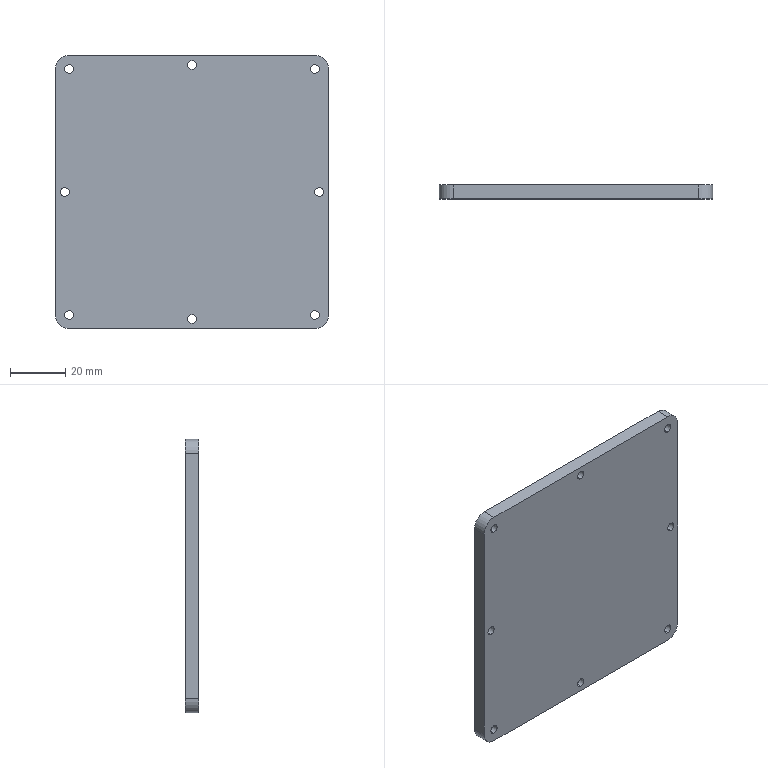Part | SolidWorks | features Extrusion 1, Fillet 1, HoleWzd 1 | 1 solid | 42 faces | box 99 x 5 x 99 mm | volume 48448 mm3 | cylinder 20 | cone 16 | plane 6 | commonest cylinder face diameters 3.2 x16 10 x4
STEP:
#1=CARTESIAN_POINT('',(-44.5,3.45,-46.1));
#2=VERTEX_POINT('',#1);
#3=CARTESIAN_POINT('',(-44.5,3.45,-42.9));
#4=VERTEX_POINT('',#3);
#5=CARTESIAN_POINT('',(-44.5,3.45,-44.5));
#6=DIRECTION('',(0.,1.,0.));
#7=DIRECTION('',(0.,0.,1.));
#8=AXIS2_PLACEMENT_3D('',#5,#6,#7);
#9=CIRCLE('',#8,1.6);
#10=EDGE_CURVE('',#2,#4,#9,.T.);
#11=ORIENTED_EDGE('',*,*,#10,.F.);
#12=CARTESIAN_POINT('',(-44.5,5.,-47.65));
#13=VERTEX_POINT('',#12);
#14=CARTESIAN_POINT('',(-44.5,5.,-47.65));
#15=DIRECTION('',(0.,0.7071,-0.7071));
#16=VECTOR('',#15,1000.);
#17=LINE('',#14,#16);
#18=EDGE_CURVE('',#2,#13,#17,.T.);
#19=ORIENTED_EDGE('',*,*,#18,.T.);
#20=CARTESIAN_POINT('',(-44.5,5.,-41.35));
#21=VERTEX_POINT('',#20);
#22=CARTESIAN_POINT('',(-44.5,5.,-44.5));
#23=DIRECTION('',(0.,1.,0.));
#24=DIRECTION('',(0.,0.,1.));
#25=AXIS2_PLACEMENT_3D('',#22,#23,#24);
#26=CIRCLE('',#25,3.15);
#27=EDGE_CURVE('',#13,#21,#26,.T.);
#28=ORIENTED_EDGE('',*,*,#27,.T.);
#29=CARTESIAN_POINT('',(-44.5,5.,-41.35));
#30=DIRECTION('',(0.,0.7071,0.7071));
#31=VECTOR('',#30,1000.);
#32=LINE('',#29,#31);
#33=EDGE_CURVE('',#4,#21,#32,.T.);
#34=ORIENTED_EDGE('',*,*,#33,.F.);
#35=EDGE_LOOP('',(#11,#19,#28,#34));
#36=FACE_OUTER_BOUND('',#35,.T.);
#37=CARTESIAN_POINT('',(-44.5,5.,-44.5));
#38=DIRECTION('',(0.,1.,0.));
#39=DIRECTION('',(0.,0.,1.));
#40=AXIS2_PLACEMENT_3D('',#37,#38,#39);
#41=CONICAL_SURFACE('',#40,3.15,0.7854);
#42=ADVANCED_FACE('',(#36),#41,.F.);
#43=CARTESIAN_POINT('',(-44.5,0.,-42.9));
#44=VERTEX_POINT('',#43);
#45=CARTESIAN_POINT('',(-44.5,0.,-46.1));
#46=VERTEX_POINT('',#45);
#47=CARTESIAN_POINT('',(-44.5,0.,-44.5));
#48=DIRECTION('',(0.,-1.,0.));
#49=DIRECTION('',(0.,0.,-1.));
#50=AXIS2_PLACEMENT_3D('',#47,#48,#49);
#51=CIRCLE('',#50,1.6);
#52=EDGE_CURVE('',#44,#46,#51,.T.);
#53=ORIENTED_EDGE('',*,*,#52,.T.);
#54=CARTESIAN_POINT('',(-44.5,5.,-46.1));
#55=DIRECTION('',(0.,1.,0.));
#56=VECTOR('',#55,1000.);
#57=LINE('',#54,#56);
#58=EDGE_CURVE('',#46,#2,#57,.T.);
#59=ORIENTED_EDGE('',*,*,#58,.T.);
#60=ORIENTED_EDGE('',*,*,#10,.T.);
#61=CARTESIAN_POINT('',(-44.5,5.,-42.9));
#62=DIRECTION('',(0.,1.,0.));
#63=VECTOR('',#62,1000.);
#64=LINE('',#61,#63);
#65=EDGE_CURVE('',#44,#4,#64,.T.);
#66=ORIENTED_EDGE('',*,*,#65,.F.);
#67=EDGE_LOOP('',(#53,#59,#60,#66));
#68=FACE_OUTER_BOUND('',#67,.T.);
#69=CARTESIAN_POINT('',(-44.5,5.,-44.5));
#70=DIRECTION('',(0.,1.,0.));
#71=DIRECTION('',(0.,0.,1.));
#72=AXIS2_PLACEMENT_3D('',#69,#70,#71);
#73=CYLINDRICAL_SURFACE('',#72,1.6);
#74=ADVANCED_FACE('',(#68),#73,.F.);
#75=CARTESIAN_POINT('',(44.5,3.45,-46.1));
#76=VERTEX_POINT('',#75);
#77=CARTESIAN_POINT('',(44.5,3.45,-42.9));
#78=VERTEX_POINT('',#77);
#79=CARTESIAN_POINT('',(44.5,3.45,-44.5));
#80=DIRECTION('',(0.,1.,0.));
#81=DIRECTION('',(0.,0.,1.));
#82=AXIS2_PLACEMENT_3D('',#79,#80,#81);
#83=CIRCLE('',#82,1.6);
#84=EDGE_CURVE('',#76,#78,#83,.T.);
#85=ORIENTED_EDGE('',*,*,#84,.F.);
#86=CARTESIAN_POINT('',(44.5,5.,-47.65));
#87=VERTEX_POINT('',#86);
#88=CARTESIAN_POINT('',(44.5,5.,-47.65));
#89=DIRECTION('',(0.,0.7071,-0.7071));
#90=VECTOR('',#89,1000.);
#91=LINE('',#88,#90);
#92=EDGE_CURVE('',#76,#87,#91,.T.);
#93=ORIENTED_EDGE('',*,*,#92,.T.);
#94=CARTESIAN_POINT('',(44.5,5.,-41.35));
#95=VERTEX_POINT('',#94);
#96=CARTESIAN_POINT('',(44.5,5.,-44.5));
#97=DIRECTION('',(0.,1.,0.));
#98=DIRECTION('',(0.,0.,1.));
#99=AXIS2_PLACEMENT_3D('',#96,#97,#98);
#100=CIRCLE('',#99,3.15);
#101=EDGE_CURVE('',#87,#95,#100,.T.);
#102=ORIENTED_EDGE('',*,*,#101,.T.);
#103=CARTESIAN_POINT('',(44.5,5.,-41.35));
#104=DIRECTION('',(0.,0.7071,0.7071));
#105=VECTOR('',#104,1000.);
#106=LINE('',#103,#105);
#107=EDGE_CURVE('',#78,#95,#106,.T.);
#108=ORIENTED_EDGE('',*,*,#107,.F.);
#109=EDGE_LOOP('',(#85,#93,#102,#108));
#110=FACE_OUTER_BOUND('',#109,.T.);
#111=CARTESIAN_POINT('',(44.5,5.,-44.5));
#112=DIRECTION('',(0.,1.,0.));
#113=DIRECTION('',(0.,0.,1.));
#114=AXIS2_PLACEMENT_3D('',#111,#112,#113);
#115=CONICAL_SURFACE('',#114,3.15,0.7854);
#116=ADVANCED_FACE('',(#110),#115,.F.);
#117=CARTESIAN_POINT('',(44.5,0.,-42.9));
#118=VERTEX_POINT('',#117);
#119=CARTESIAN_POINT('',(44.5,0.,-46.1));
#120=VERTEX_POINT('',#119);
#121=CARTESIAN_POINT('',(44.5,0.,-44.5));
#122=DIRECTION('',(0.,-1.,0.));
#123=DIRECTION('',(0.,0.,-1.));
#124=AXIS2_PLACEMENT_3D('',#121,#122,#123);
#125=CIRCLE('',#124,1.6);
#126=EDGE_CURVE('',#118,#120,#125,.T.);
#127=ORIENTED_EDGE('',*,*,#126,.T.);
#128=CARTESIAN_POINT('',(44.5,5.,-46.1));
#129=DIRECTION('',(0.,1.,0.));
#130=VECTOR('',#129,1000.);
#131=LINE('',#128,#130);
#132=EDGE_CURVE('',#120,#76,#131,.T.);
#133=ORIENTED_EDGE('',*,*,#132,.T.);
#134=ORIENTED_EDGE('',*,*,#84,.T.);
#135=CARTESIAN_POINT('',(44.5,5.,-42.9));
#136=DIRECTION('',(0.,1.,0.));
#137=VECTOR('',#136,1000.);
#138=LINE('',#135,#137);
#139=EDGE_CURVE('',#118,#78,#138,.T.);
#140=ORIENTED_EDGE('',*,*,#139,.F.);
#141=EDGE_LOOP('',(#127,#133,#134,#140));
#142=FACE_OUTER_BOUND('',#141,.T.);
#143=CARTESIAN_POINT('',(44.5,5.,-44.5));
#144=DIRECTION('',(0.,1.,0.));
#145=DIRECTION('',(0.,0.,1.));
#146=AXIS2_PLACEMENT_3D('',#143,#144,#145);
#147=CYLINDRICAL_SURFACE('',#146,1.6);
#148=ADVANCED_FACE('',(#142),#147,.F.);
#149=CARTESIAN_POINT('',(0.,3.45,-47.6));
#150=VERTEX_POINT('',#149);
#151=CARTESIAN_POINT('',(0.,3.45,-44.4));
#152=VERTEX_POINT('',#151);
#153=CARTESIAN_POINT('',(0.,3.45,-46.));
#154=DIRECTION('',(0.,1.,0.));
#155=DIRECTION('',(0.,0.,1.));
#156=AXIS2_PLACEMENT_3D('',#153,#154,#155);
#157=CIRCLE('',#156,1.6);
#158=EDGE_CURVE('',#150,#152,#157,.T.);
#159=ORIENTED_EDGE('',*,*,#158,.F.);
#160=CARTESIAN_POINT('',(0.,5.,-49.15));
#161=VERTEX_POINT('',#160);
#162=CARTESIAN_POINT('',(0.,5.,-49.15));
#163=DIRECTION('',(0.,0.7071,-0.7071));
#164=VECTOR('',#163,1000.);
#165=LINE('',#162,#164);
#166=EDGE_CURVE('',#150,#161,#165,.T.);
#167=ORIENTED_EDGE('',*,*,#166,.T.);
#168=CARTESIAN_POINT('',(0.,5.,-42.85));
#169=VERTEX_POINT('',#168);
#170=CARTESIAN_POINT('',(0.,5.,-46.));
#171=DIRECTION('',(0.,1.,0.));
#172=DIRECTION('',(0.,0.,1.));
#173=AXIS2_PLACEMENT_3D('',#170,#171,#172);
#174=CIRCLE('',#173,3.15);
#175=EDGE_CURVE('',#161,#169,#174,.T.);
#176=ORIENTED_EDGE('',*,*,#175,.T.);
#177=CARTESIAN_POINT('',(0.,5.,-42.85));
#178=DIRECTION('',(0.,0.7071,0.7071));
#179=VECTOR('',#178,1000.);
#180=LINE('',#177,#179);
#181=EDGE_CURVE('',#152,#169,#180,.T.);
#182=ORIENTED_EDGE('',*,*,#181,.F.);
#183=EDGE_LOOP('',(#159,#167,#176,#182));
#184=FACE_OUTER_BOUND('',#183,.T.);
#185=CARTESIAN_POINT('',(0.,5.,-46.));
#186=DIRECTION('',(0.,1.,0.));
#187=DIRECTION('',(0.,0.,1.));
#188=AXIS2_PLACEMENT_3D('',#185,#186,#187);
#189=CONICAL_SURFACE('',#188,3.15,0.7854);
#190=ADVANCED_FACE('',(#184),#189,.F.);
#191=CARTESIAN_POINT('',(0.,0.,-44.4));
#192=VERTEX_POINT('',#191);
#193=CARTESIAN_POINT('',(0.,0.,-47.6));
#194=VERTEX_POINT('',#193);
#195=CARTESIAN_POINT('',(0.,0.,-46.));
#196=DIRECTION('',(0.,-1.,0.));
#197=DIRECTION('',(0.,0.,-1.));
#198=AXIS2_PLACEMENT_3D('',#195,#196,#197);
#199=CIRCLE('',#198,1.6);
#200=EDGE_CURVE('',#192,#194,#199,.T.);
#201=ORIENTED_EDGE('',*,*,#200,.T.);
#202=CARTESIAN_POINT('',(0.,5.,-47.6));
#203=DIRECTION('',(0.,1.,0.));
#204=VECTOR('',#203,1000.);
#205=LINE('',#202,#204);
#206=EDGE_CURVE('',#194,#150,#205,.T.);
#207=ORIENTED_EDGE('',*,*,#206,.T.);
#208=ORIENTED_EDGE('',*,*,#158,.T.);
#209=CARTESIAN_POINT('',(0.,5.,-44.4));
#210=DIRECTION('',(0.,1.,0.));
#211=VECTOR('',#210,1000.);
#212=LINE('',#209,#211);
#213=EDGE_CURVE('',#192,#152,#212,.T.);
#214=ORIENTED_EDGE('',*,*,#213,.F.);
#215=EDGE_LOOP('',(#201,#207,#208,#214));
#216=FACE_OUTER_BOUND('',#215,.T.);
#217=CARTESIAN_POINT('',(0.,5.,-46.));
#218=DIRECTION('',(0.,1.,0.));
#219=DIRECTION('',(0.,0.,1.));
#220=AXIS2_PLACEMENT_3D('',#217,#218,#219);
#221=CYLINDRICAL_SURFACE('',#220,1.6);
#222=ADVANCED_FACE('',(#216),#221,.F.);
#223=CARTESIAN_POINT('',(-46.,3.45,-1.6));
#224=VERTEX_POINT('',#223);
#225=CARTESIAN_POINT('',(-46.,3.45,1.6));
#226=VERTEX_POINT('',#225);
#227=CARTESIAN_POINT('',(-46.,3.45,0.));
#228=DIRECTION('',(0.,1.,0.));
#229=DIRECTION('',(0.,0.,1.));
#230=AXIS2_PLACEMENT_3D('',#227,#228,#229);
#231=CIRCLE('',#230,1.6);
#232=EDGE_CURVE('',#224,#226,#231,.T.);
#233=ORIENTED_EDGE('',*,*,#232,.F.);
#234=CARTESIAN_POINT('',(-46.,5.,-3.15));
#235=VERTEX_POINT('',#234);
#236=CARTESIAN_POINT('',(-46.,5.,-3.15));
#237=DIRECTION('',(0.,0.7071,-0.7071));
#238=VECTOR('',#237,1000.);
#239=LINE('',#236,#238);
#240=EDGE_CURVE('',#224,#235,#239,.T.);
#241=ORIENTED_EDGE('',*,*,#240,.T.);
#242=CARTESIAN_POINT('',(-46.,5.,3.15));
#243=VERTEX_POINT('',#242);
#244=CARTESIAN_POINT('',(-46.,5.,0.));
#245=DIRECTION('',(0.,1.,0.));
#246=DIRECTION('',(0.,0.,1.));
#247=AXIS2_PLACEMENT_3D('',#244,#245,#246);
#248=CIRCLE('',#247,3.15);
#249=EDGE_CURVE('',#235,#243,#248,.T.);
#250=ORIENTED_EDGE('',*,*,#249,.T.);
#251=CARTESIAN_POINT('',(-46.,5.,3.15));
#252=DIRECTION('',(0.,0.7071,0.7071));
#253=VECTOR('',#252,1000.);
#254=LINE('',#251,#253);
#255=EDGE_CURVE('',#226,#243,#254,.T.);
#256=ORIENTED_EDGE('',*,*,#255,.F.);
#257=EDGE_LOOP('',(#233,#241,#250,#256));
#258=FACE_OUTER_BOUND('',#257,.T.);
#259=CARTESIAN_POINT('',(-46.,5.,0.));
#260=DIRECTION('',(0.,1.,0.));
#261=DIRECTION('',(0.,0.,1.));
#262=AXIS2_PLACEMENT_3D('',#259,#260,#261);
#263=CONICAL_SURFACE('',#262,3.15,0.7854);
#264=ADVANCED_FACE('',(#258),#263,.F.);
#265=CARTESIAN_POINT('',(-46.,0.,1.6));
#266=VERTEX_POINT('',#265);
#267=CARTESIAN_POINT('',(-46.,0.,-1.6));
#268=VERTEX_POINT('',#267);
#269=CARTESIAN_POINT('',(-46.,0.,0.));
#270=DIRECTION('',(0.,-1.,0.));
#271=DIRECTION('',(0.,0.,-1.));
#272=AXIS2_PLACEMENT_3D('',#269,#270,#271);
#273=CIRCLE('',#272,1.6);
#274=EDGE_CURVE('',#266,#268,#273,.T.);
#275=ORIENTED_EDGE('',*,*,#274,.T.);
#276=CARTESIAN_POINT('',(-46.,5.,-1.6));
#277=DIRECTION('',(0.,1.,0.));
#278=VECTOR('',#277,1000.);
#279=LINE('',#276,#278);
#280=EDGE_CURVE('',#268,#224,#279,.T.);
#281=ORIENTED_EDGE('',*,*,#280,.T.);
#282=ORIENTED_EDGE('',*,*,#232,.T.);
#283=CARTESIAN_POINT('',(-46.,5.,1.6));
#284=DIRECTION('',(0.,1.,0.));
#285=VECTOR('',#284,1000.);
#286=LINE('',#283,#285);
#287=EDGE_CURVE('',#266,#226,#286,.T.);
#288=ORIENTED_EDGE('',*,*,#287,.F.);
#289=EDGE_LOOP('',(#275,#281,#282,#288));
#290=FACE_OUTER_BOUND('',#289,.T.);
#291=CARTESIAN_POINT('',(-46.,5.,0.));
#292=DIRECTION('',(0.,1.,0.));
#293=DIRECTION('',(0.,0.,1.));
#294=AXIS2_PLACEMENT_3D('',#291,#292,#293);
#295=CYLINDRICAL_SURFACE('',#294,1.6);
#296=ADVANCED_FACE('',(#290),#295,.F.);
#297=CARTESIAN_POINT('',(-44.5,3.45,42.9));
#298=VERTEX_POINT('',#297);
#299=CARTESIAN_POINT('',(-44.5,3.45,46.1));
#300=VERTEX_POINT('',#299);
#301=CARTESIAN_POINT('',(-44.5,3.45,44.5));
#302=DIRECTION('',(0.,1.,0.));
#303=DIRECTION('',(0.,0.,1.));
#304=AXIS2_PLACEMENT_3D('',#301,#302,#303);
#305=CIRCLE('',#304,1.6);
#306=EDGE_CURVE('',#298,#300,#305,.T.);
#307=ORIENTED_EDGE('',*,*,#306,.F.);
#308=CARTESIAN_POINT('',(-44.5,5.,41.35));
#309=VERTEX_POINT('',#308);
#310=CARTESIAN_POINT('',(-44.5,5.,41.35));
#311=DIRECTION('',(0.,0.7071,-0.7071));
#312=VECTOR('',#311,1000.);
#313=LINE('',#310,#312);
#314=EDGE_CURVE('',#298,#309,#313,.T.);
#315=ORIENTED_EDGE('',*,*,#314,.T.);
#316=CARTESIAN_POINT('',(-44.5,5.,47.65));
#317=VERTEX_POINT('',#316);
#318=CARTESIAN_POINT('',(-44.5,5.,44.5));
#319=DIRECTION('',(0.,1.,0.));
#320=DIRECTION('',(0.,0.,1.));
#321=AXIS2_PLACEMENT_3D('',#318,#319,#320);
#322=CIRCLE('',#321,3.15);
#323=EDGE_CURVE('',#309,#317,#322,.T.);
#324=ORIENTED_EDGE('',*,*,#323,.T.);
#325=CARTESIAN_POINT('',(-44.5,5.,47.65));
#326=DIRECTION('',(0.,0.7071,0.7071));
#327=VECTOR('',#326,1000.);
#328=LINE('',#325,#327);
#329=EDGE_CURVE('',#300,#317,#328,.T.);
#330=ORIENTED_EDGE('',*,*,#329,.F.);
#331=EDGE_LOOP('',(#307,#315,#324,#330));
#332=FACE_OUTER_BOUND('',#331,.T.);
#333=CARTESIAN_POINT('',(-44.5,5.,44.5));
#334=DIRECTION('',(0.,1.,0.));
#335=DIRECTION('',(0.,0.,1.));
#336=AXIS2_PLACEMENT_3D('',#333,#334,#335);
#337=CONICAL_SURFACE('',#336,3.15,0.7854);
#338=ADVANCED_FACE('',(#332),#337,.F.);
#339=CARTESIAN_POINT('',(-44.5,0.,46.1));
#340=VERTEX_POINT('',#339);
#341=CARTESIAN_POINT('',(-44.5,0.,42.9));
#342=VERTEX_POINT('',#341);
#343=CARTESIAN_POINT('',(-44.5,0.,44.5));
#344=DIRECTION('',(0.,-1.,0.));
#345=DIRECTION('',(0.,0.,-1.));
#346=AXIS2_PLACEMENT_3D('',#343,#344,#345);
#347=CIRCLE('',#346,1.6);
#348=EDGE_CURVE('',#340,#342,#347,.T.);
#349=ORIENTED_EDGE('',*,*,#348,.T.);
#350=CARTESIAN_POINT('',(-44.5,5.,42.9));
#351=DIRECTION('',(0.,1.,0.));
#352=VECTOR('',#351,1000.);
#353=LINE('',#350,#352);
#354=EDGE_CURVE('',#342,#298,#353,.T.);
#355=ORIENTED_EDGE('',*,*,#354,.T.);
#356=ORIENTED_EDGE('',*,*,#306,.T.);
#357=CARTESIAN_POINT('',(-44.5,5.,46.1));
#358=DIRECTION('',(0.,1.,0.));
#359=VECTOR('',#358,1000.);
#360=LINE('',#357,#359);
#361=EDGE_CURVE('',#340,#300,#360,.T.);
#362=ORIENTED_EDGE('',*,*,#361,.F.);
#363=EDGE_LOOP('',(#349,#355,#356,#362));
#364=FACE_OUTER_BOUND('',#363,.T.);
#365=CARTESIAN_POINT('',(-44.5,5.,44.5));
#366=DIRECTION('',(0.,1.,0.));
#367=DIRECTION('',(0.,0.,1.));
#368=AXIS2_PLACEMENT_3D('',#365,#366,#367);
#369=CYLINDRICAL_SURFACE('',#368,1.6);
#370=ADVANCED_FACE('',(#364),#369,.F.);
#371=CARTESIAN_POINT('',(0.,3.45,44.4));
#372=VERTEX_POINT('',#371);
#373=CARTESIAN_POINT('',(0.,3.45,47.6));
#374=VERTEX_POINT('',#373);
#375=CARTESIAN_POINT('',(0.,3.45,46.));
#376=DIRECTION('',(0.,1.,0.));
#377=DIRECTION('',(0.,0.,1.));
#378=AXIS2_PLACEMENT_3D('',#375,#376,#377);
#379=CIRCLE('',#378,1.6);
#380=EDGE_CURVE('',#372,#374,#379,.T.);
#381=ORIENTED_EDGE('',*,*,#380,.F.);
#382=CARTESIAN_POINT('',(0.,5.,42.85));
#383=VERTEX_POINT('',#382);
#384=CARTESIAN_POINT('',(0.,5.,42.85));
#385=DIRECTION('',(0.,0.7071,-0.7071));
#386=VECTOR('',#385,1000.);
#387=LINE('',#384,#386);
#388=EDGE_CURVE('',#372,#383,#387,.T.);
#389=ORIENTED_EDGE('',*,*,#388,.T.);
#390=CARTESIAN_POINT('',(0.,5.,49.15));
#391=VERTEX_POINT('',#390);
#392=CARTESIAN_POINT('',(0.,5.,46.));
#393=DIRECTION('',(0.,1.,0.));
#394=DIRECTION('',(0.,0.,1.));
#395=AXIS2_PLACEMENT_3D('',#392,#393,#394);
#396=CIRCLE('',#395,3.15);
#397=EDGE_CURVE('',#383,#391,#396,.T.);
#398=ORIENTED_EDGE('',*,*,#397,.T.);
#399=CARTESIAN_POINT('',(0.,5.,49.15));
#400=DIRECTION('',(0.,0.7071,0.7071));
#401=VECTOR('',#400,1000.);
#402=LINE('',#399,#401);
#403=EDGE_CURVE('',#374,#391,#402,.T.);
#404=ORIENTED_EDGE('',*,*,#403,.F.);
#405=EDGE_LOOP('',(#381,#389,#398,#404));
#406=FACE_OUTER_BOUND('',#405,.T.);
#407=CARTESIAN_POINT('',(0.,5.,46.));
#408=DIRECTION('',(0.,1.,0.));
#409=DIRECTION('',(0.,0.,1.));
#410=AXIS2_PLACEMENT_3D('',#407,#408,#409);
#411=CONICAL_SURFACE('',#410,3.15,0.7854);
#412=ADVANCED_FACE('',(#406),#411,.F.);
#413=CARTESIAN_POINT('',(0.,0.,47.6));
#414=VERTEX_POINT('',#413);
#415=CARTESIAN_POINT('',(0.,0.,44.4));
#416=VERTEX_POINT('',#415);
#417=CARTESIAN_POINT('',(0.,0.,46.));
#418=DIRECTION('',(0.,-1.,0.));
#419=DIRECTION('',(0.,0.,-1.));
#420=AXIS2_PLACEMENT_3D('',#417,#418,#419);
#421=CIRCLE('',#420,1.6);
#422=EDGE_CURVE('',#414,#416,#421,.T.);
#423=ORIENTED_EDGE('',*,*,#422,.T.);
#424=CARTESIAN_POINT('',(0.,5.,44.4));
#425=DIRECTION('',(0.,1.,0.));
#426=VECTOR('',#425,1000.);
#427=LINE('',#424,#426);
#428=EDGE_CURVE('',#416,#372,#427,.T.);
#429=ORIENTED_EDGE('',*,*,#428,.T.);
#430=ORIENTED_EDGE('',*,*,#380,.T.);
#431=CARTESIAN_POINT('',(0.,5.,47.6));
#432=DIRECTION('',(0.,1.,0.));
#433=VECTOR('',#432,1000.);
#434=LINE('',#431,#433);
#435=EDGE_CURVE('',#414,#374,#434,.T.);
#436=ORIENTED_EDGE('',*,*,#435,.F.);
#437=EDGE_LOOP('',(#423,#429,#430,#436));
#438=FACE_OUTER_BOUND('',#437,.T.);
#439=CARTESIAN_POINT('',(0.,5.,46.));
#440=DIRECTION('',(0.,1.,0.));
#441=DIRECTION('',(0.,0.,1.));
#442=AXIS2_PLACEMENT_3D('',#439,#440,#441);
#443=CYLINDRICAL_SURFACE('',#442,1.6);
#444=ADVANCED_FACE('',(#438),#443,.F.);
#445=CARTESIAN_POINT('',(44.5,3.45,42.9));
#446=VERTEX_POINT('',#445);
#447=CARTESIAN_POINT('',(44.5,3.45,46.1));
#448=VERTEX_POINT('',#447);
#449=CARTESIAN_POINT('',(44.5,3.45,44.5));
#450=DIRECTION('',(0.,1.,0.));
#451=DIRECTION('',(0.,0.,1.));
#452=AXIS2_PLACEMENT_3D('',#449,#450,#451);
#453=CIRCLE('',#452,1.6);
#454=EDGE_CURVE('',#446,#448,#453,.T.);
#455=ORIENTED_EDGE('',*,*,#454,.F.);
#456=CARTESIAN_POINT('',(44.5,5.,41.35));
#457=VERTEX_POINT('',#456);
#458=CARTESIAN_POINT('',(44.5,5.,41.35));
#459=DIRECTION('',(0.,0.7071,-0.7071));
#460=VECTOR('',#459,1000.);
#461=LINE('',#458,#460);
#462=EDGE_CURVE('',#446,#457,#461,.T.);
#463=ORIENTED_EDGE('',*,*,#462,.T.);
#464=CARTESIAN_POINT('',(44.5,5.,47.65));
#465=VERTEX_POINT('',#464);
#466=CARTESIAN_POINT('',(44.5,5.,44.5));
#467=DIRECTION('',(0.,1.,0.));
#468=DIRECTION('',(0.,0.,1.));
#469=AXIS2_PLACEMENT_3D('',#466,#467,#468);
#470=CIRCLE('',#469,3.15);
#471=EDGE_CURVE('',#457,#465,#470,.T.);
#472=ORIENTED_EDGE('',*,*,#471,.T.);
#473=CARTESIAN_POINT('',(44.5,5.,47.65));
#474=DIRECTION('',(0.,0.7071,0.7071));
#475=VECTOR('',#474,1000.);
#476=LINE('',#473,#475);
#477=EDGE_CURVE('',#448,#465,#476,.T.);
#478=ORIENTED_EDGE('',*,*,#477,.F.);
#479=EDGE_LOOP('',(#455,#463,#472,#478));
#480=FACE_OUTER_BOUND('',#479,.T.);
#481=CARTESIAN_POINT('',(44.5,5.,44.5));
#482=DIRECTION('',(0.,1.,0.));
#483=DIRECTION('',(0.,0.,1.));
#484=AXIS2_PLACEMENT_3D('',#481,#482,#483);
#485=CONICAL_SURFACE('',#484,3.15,0.7854);
#486=ADVANCED_FACE('',(#480),#485,.F.);
#487=CARTESIAN_POINT('',(44.5,0.,46.1));
#488=VERTEX_POINT('',#487);
#489=CARTESIAN_POINT('',(44.5,0.,42.9));
#490=VERTEX_POINT('',#489);
#491=CARTESIAN_POINT('',(44.5,0.,44.5));
#492=DIRECTION('',(0.,-1.,0.));
#493=DIRECTION('',(0.,0.,-1.));
#494=AXIS2_PLACEMENT_3D('',#491,#492,#493);
#495=CIRCLE('',#494,1.6);
#496=EDGE_CURVE('',#488,#490,#495,.T.);
#497=ORIENTED_EDGE('',*,*,#496,.T.);
#498=CARTESIAN_POINT('',(44.5,5.,42.9));
#499=DIRECTION('',(0.,1.,0.));
#500=VECTOR('',#499,1000.);
#501=LINE('',#498,#500);
#502=EDGE_CURVE('',#490,#446,#501,.T.);
#503=ORIENTED_EDGE('',*,*,#502,.T.);
#504=ORIENTED_EDGE('',*,*,#454,.T.);
#505=CARTESIAN_POINT('',(44.5,5.,46.1));
#506=DIRECTION('',(0.,1.,0.));
#507=VECTOR('',#506,1000.);
#508=LINE('',#505,#507);
#509=EDGE_CURVE('',#488,#448,#508,.T.);
#510=ORIENTED_EDGE('',*,*,#509,.F.);
#511=EDGE_LOOP('',(#497,#503,#504,#510));
#512=FACE_OUTER_BOUND('',#511,.T.);
#513=CARTESIAN_POINT('',(44.5,5.,44.5));
#514=DIRECTION('',(0.,1.,0.));
#515=DIRECTION('',(0.,0.,1.));
#516=AXIS2_PLACEMENT_3D('',#513,#514,#515);
#517=CYLINDRICAL_SURFACE('',#516,1.6);
#518=ADVANCED_FACE('',(#512),#517,.F.);
#519=CARTESIAN_POINT('',(46.,3.45,-1.6));
#520=VERTEX_POINT('',#519);
#521=CARTESIAN_POINT('',(46.,3.45,1.6));
#522=VERTEX_POINT('',#521);
#523=CARTESIAN_POINT('',(46.,3.45,0.));
#524=DIRECTION('',(0.,1.,0.));
#525=DIRECTION('',(0.,0.,1.));
#526=AXIS2_PLACEMENT_3D('',#523,#524,#525);
#527=CIRCLE('',#526,1.6);
#528=EDGE_CURVE('',#520,#522,#527,.T.);
#529=ORIENTED_EDGE('',*,*,#528,.F.);
#530=CARTESIAN_POINT('',(46.,5.,-3.15));
#531=VERTEX_POINT('',#530);
#532=CARTESIAN_POINT('',(46.,5.,-3.15));
#533=DIRECTION('',(0.,0.7071,-0.7071));
#534=VECTOR('',#533,1000.);
#535=LINE('',#532,#534);
#536=EDGE_CURVE('',#520,#531,#535,.T.);
#537=ORIENTED_EDGE('',*,*,#536,.T.);
#538=CARTESIAN_POINT('',(46.,5.,3.15));
#539=VERTEX_POINT('',#538);
#540=CARTESIAN_POINT('',(46.,5.,0.));
#541=DIRECTION('',(0.,1.,0.));
#542=DIRECTION('',(0.,0.,1.));
#543=AXIS2_PLACEMENT_3D('',#540,#541,#542);
#544=CIRCLE('',#543,3.15);
#545=EDGE_CURVE('',#531,#539,#544,.T.);
#546=ORIENTED_EDGE('',*,*,#545,.T.);
#547=CARTESIAN_POINT('',(46.,5.,3.15));
#548=DIRECTION('',(0.,0.7071,0.7071));
#549=VECTOR('',#548,1000.);
#550=LINE('',#547,#549);
#551=EDGE_CURVE('',#522,#539,#550,.T.);
#552=ORIENTED_EDGE('',*,*,#551,.F.);
#553=EDGE_LOOP('',(#529,#537,#546,#552));
#554=FACE_OUTER_BOUND('',#553,.T.);
#555=CARTESIAN_POINT('',(46.,5.,0.));
#556=DIRECTION('',(0.,1.,0.));
#557=DIRECTION('',(0.,0.,1.));
#558=AXIS2_PLACEMENT_3D('',#555,#556,#557);
#559=CONICAL_SURFACE('',#558,3.15,0.7854);
#560=ADVANCED_FACE('',(#554),#559,.F.);
#561=CARTESIAN_POINT('',(46.,0.,1.6));
#562=VERTEX_POINT('',#561);
#563=CARTESIAN_POINT('',(46.,0.,-1.6));
#564=VERTEX_POINT('',#563);
#565=CARTESIAN_POINT('',(46.,0.,0.));
#566=DIRECTION('',(0.,-1.,0.));
#567=DIRECTION('',(0.,0.,-1.));
#568=AXIS2_PLACEMENT_3D('',#565,#566,#567);
#569=CIRCLE('',#568,1.6);
#570=EDGE_CURVE('',#562,#564,#569,.T.);
#571=ORIENTED_EDGE('',*,*,#570,.T.);
#572=CARTESIAN_POINT('',(46.,5.,-1.6));
#573=DIRECTION('',(0.,1.,0.));
#574=VECTOR('',#573,1000.);
#575=LINE('',#572,#574);
#576=EDGE_CURVE('',#564,#520,#575,.T.);
#577=ORIENTED_EDGE('',*,*,#576,.T.);
#578=ORIENTED_EDGE('',*,*,#528,.T.);
#579=CARTESIAN_POINT('',(46.,5.,1.6));
#580=DIRECTION('',(0.,1.,0.));
#581=VECTOR('',#580,1000.);
#582=LINE('',#579,#581);
#583=EDGE_CURVE('',#562,#522,#582,.T.);
#584=ORIENTED_EDGE('',*,*,#583,.F.);
#585=EDGE_LOOP('',(#571,#577,#578,#584));
#586=FACE_OUTER_BOUND('',#585,.T.);
#587=CARTESIAN_POINT('',(46.,5.,0.));
#588=DIRECTION('',(0.,1.,0.));
#589=DIRECTION('',(0.,0.,1.));
#590=AXIS2_PLACEMENT_3D('',#587,#588,#589);
#591=CYLINDRICAL_SURFACE('',#590,1.6);
#592=ADVANCED_FACE('',(#586),#591,.F.);
#593=CARTESIAN_POINT('',(-44.5,5.,-44.5));
#594=DIRECTION('',(0.,1.,0.));
#595=DIRECTION('',(0.,0.,1.));
#596=AXIS2_PLACEMENT_3D('',#593,#594,#595);
#597=CIRCLE('',#596,3.15);
#598=EDGE_CURVE('',#21,#13,#597,.T.);
#599=ORIENTED_EDGE('',*,*,#598,.F.);
#600=ORIENTED_EDGE('',*,*,#27,.F.);
#601=EDGE_LOOP('',(#599,#600));
#602=FACE_BOUND('',#601,.T.);
#603=CARTESIAN_POINT('',(44.5,5.,-44.5));
#604=DIRECTION('',(0.,1.,0.));
#605=DIRECTION('',(0.,0.,1.));
#606=AXIS2_PLACEMENT_3D('',#603,#604,#605);
#607=CIRCLE('',#606,3.15);
#608=EDGE_CURVE('',#95,#87,#607,.T.);
#609=ORIENTED_EDGE('',*,*,#608,.F.);
#610=ORIENTED_EDGE('',*,*,#101,.F.);
#611=EDGE_LOOP('',(#609,#610));
#612=FACE_BOUND('',#611,.T.);
#613=CARTESIAN_POINT('',(-44.5,5.,44.5));
#614=DIRECTION('',(0.,1.,0.));
#615=DIRECTION('',(0.,0.,1.));
#616=AXIS2_PLACEMENT_3D('',#613,#614,#615);
#617=CIRCLE('',#616,3.15);
#618=EDGE_CURVE('',#317,#309,#617,.T.);
#619=ORIENTED_EDGE('',*,*,#618,.F.);
#620=ORIENTED_EDGE('',*,*,#323,.F.);
#621=EDGE_LOOP('',(#619,#620));
#622=FACE_BOUND('',#621,.T.);
#623=CARTESIAN_POINT('',(0.,5.,46.));
#624=DIRECTION('',(0.,1.,0.));
#625=DIRECTION('',(0.,0.,1.));
#626=AXIS2_PLACEMENT_3D('',#623,#624,#625);
#627=CIRCLE('',#626,3.15);
#628=EDGE_CURVE('',#391,#383,#627,.T.);
#629=ORIENTED_EDGE('',*,*,#628,.F.);
#630=ORIENTED_EDGE('',*,*,#397,.F.);
#631=EDGE_LOOP('',(#629,#630));
#632=FACE_BOUND('',#631,.T.);
#633=CARTESIAN_POINT('',(44.5,5.,44.5));
#634=DIRECTION('',(0.,1.,0.));
#635=DIRECTION('',(0.,0.,1.));
#636=AXIS2_PLACEMENT_3D('',#633,#634,#635);
#637=CIRCLE('',#636,3.15);
#638=EDGE_CURVE('',#465,#457,#637,.T.);
#639=ORIENTED_EDGE('',*,*,#638,.F.);
#640=ORIENTED_EDGE('',*,*,#471,.F.);
#641=EDGE_LOOP('',(#639,#640));
#642=FACE_BOUND('',#641,.T.);
#643=CARTESIAN_POINT('',(46.,5.,0.));
#644=DIRECTION('',(0.,1.,0.));
#645=DIRECTION('',(0.,0.,1.));
#646=AXIS2_PLACEMENT_3D('',#643,#644,#645);
#647=CIRCLE('',#646,3.15);
#648=EDGE_CURVE('',#539,#531,#647,.T.);
#649=ORIENTED_EDGE('',*,*,#648,.F.);
#650=ORIENTED_EDGE('',*,*,#545,.F.);
#651=EDGE_LOOP('',(#649,#650));
#652=FACE_BOUND('',#651,.T.);
#653=CARTESIAN_POINT('',(-49.5,5.,-44.5));
#654=VERTEX_POINT('',#653);
#655=CARTESIAN_POINT('',(-49.5,5.,44.5));
#656=VERTEX_POINT('',#655);
#657=CARTESIAN_POINT('',(-49.5,5.,49.5));
#658=DIRECTION('',(0.,0.,1.));
#659=VECTOR('',#658,1000.);
#660=LINE('',#657,#659);
#661=EDGE_CURVE('',#654,#656,#660,.T.);
#662=ORIENTED_EDGE('',*,*,#661,.T.);
#663=CARTESIAN_POINT('',(-44.5,5.,49.5));
#664=VERTEX_POINT('',#663);
#665=CARTESIAN_POINT('',(-44.5,5.,44.5));
#666=DIRECTION('',(0.,1.,0.));
#667=DIRECTION('',(0.,0.,-1.));
#668=AXIS2_PLACEMENT_3D('',#665,#666,#667);
#669=CIRCLE('',#668,5.);
#670=EDGE_CURVE('',#656,#664,#669,.T.);
#671=ORIENTED_EDGE('',*,*,#670,.T.);
#672=CARTESIAN_POINT('',(44.5,5.,49.5));
#673=VERTEX_POINT('',#672);
#674=CARTESIAN_POINT('',(-49.5,5.,49.5));
#675=DIRECTION('',(1.,0.,0.));
#676=VECTOR('',#675,1000.);
#677=LINE('',#674,#676);
#678=EDGE_CURVE('',#664,#673,#677,.T.);
#679=ORIENTED_EDGE('',*,*,#678,.T.);
#680=CARTESIAN_POINT('',(49.5,5.,44.5));
#681=VERTEX_POINT('',#680);
#682=CARTESIAN_POINT('',(44.5,5.,44.5));
#683=DIRECTION('',(0.,1.,0.));
#684=DIRECTION('',(0.,0.,-1.));
#685=AXIS2_PLACEMENT_3D('',#682,#683,#684);
#686=CIRCLE('',#685,5.);
#687=EDGE_CURVE('',#673,#681,#686,.T.);
#688=ORIENTED_EDGE('',*,*,#687,.T.);
#689=CARTESIAN_POINT('',(49.5,5.,-44.5));
#690=VERTEX_POINT('',#689);
#691=CARTESIAN_POINT('',(49.5,5.,49.5));
#692=DIRECTION('',(0.,0.,-1.));
#693=VECTOR('',#692,1000.);
#694=LINE('',#691,#693);
#695=EDGE_CURVE('',#681,#690,#694,.T.);
#696=ORIENTED_EDGE('',*,*,#695,.T.);
#697=CARTESIAN_POINT('',(44.5,5.,-49.5));
#698=VERTEX_POINT('',#697);
#699=CARTESIAN_POINT('',(44.5,5.,-44.5));
#700=DIRECTION('',(0.,1.,0.));
#701=DIRECTION('',(0.,0.,-1.));
#702=AXIS2_PLACEMENT_3D('',#699,#700,#701);
#703=CIRCLE('',#702,5.);
#704=EDGE_CURVE('',#690,#698,#703,.T.);
#705=ORIENTED_EDGE('',*,*,#704,.T.);
#706=CARTESIAN_POINT('',(-44.5,5.,-49.5));
#707=VERTEX_POINT('',#706);
#708=CARTESIAN_POINT('',(-49.5,5.,-49.5));
#709=DIRECTION('',(-1.,0.,0.));
#710=VECTOR('',#709,1000.);
#711=LINE('',#708,#710);
#712=EDGE_CURVE('',#698,#707,#711,.T.);
#713=ORIENTED_EDGE('',*,*,#712,.T.);
#714=CARTESIAN_POINT('',(-44.5,5.,-44.5));
#715=DIRECTION('',(0.,1.,0.));
#716=DIRECTION('',(0.,0.,-1.));
#717=AXIS2_PLACEMENT_3D('',#714,#715,#716);
#718=CIRCLE('',#717,5.);
#719=EDGE_CURVE('',#707,#654,#718,.T.);
#720=ORIENTED_EDGE('',*,*,#719,.T.);
#721=EDGE_LOOP('',(#662,#671,#679,#688,#696,#705,#713,#720));
#722=FACE_OUTER_BOUND('',#721,.T.);
#723=CARTESIAN_POINT('',(-46.,5.,0.));
#724=DIRECTION('',(0.,1.,0.));
#725=DIRECTION('',(0.,0.,1.));
#726=AXIS2_PLACEMENT_3D('',#723,#724,#725);
#727=CIRCLE('',#726,3.15);
#728=EDGE_CURVE('',#243,#235,#727,.T.);
#729=ORIENTED_EDGE('',*,*,#728,.F.);
#730=ORIENTED_EDGE('',*,*,#249,.F.);
#731=EDGE_LOOP('',(#729,#730));
#732=FACE_BOUND('',#731,.T.);
#733=CARTESIAN_POINT('',(0.,5.,-46.));
#734=DIRECTION('',(0.,1.,0.));
#735=DIRECTION('',(0.,0.,1.));
#736=AXIS2_PLACEMENT_3D('',#733,#734,#735);
#737=CIRCLE('',#736,3.15);
#738=EDGE_CURVE('',#169,#161,#737,.T.);
#739=ORIENTED_EDGE('',*,*,#738,.F.);
#740=ORIENTED_EDGE('',*,*,#175,.F.);
#741=EDGE_LOOP('',(#739,#740));
#742=FACE_BOUND('',#741,.T.);
#743=CARTESIAN_POINT('',(0.,5.,0.));
#744=DIRECTION('',(0.,-1.,0.));
#745=DIRECTION('',(0.,0.,-1.));
#746=AXIS2_PLACEMENT_3D('',#743,#744,#745);
#747=PLANE('',#746);
#748=ADVANCED_FACE('',(#602,#612,#622,#632,#642,#652,#722,#732,#742),#747,.F.);
#749=ORIENTED_EDGE('',*,*,#695,.F.);
#750=CARTESIAN_POINT('',(49.5,0.,44.5));
#751=VERTEX_POINT('',#750);
#752=CARTESIAN_POINT('',(49.5,5.,44.5));
#753=DIRECTION('',(0.,-1.,0.));
#754=VECTOR('',#753,1000.);
#755=LINE('',#752,#754);
#756=EDGE_CURVE('',#681,#751,#755,.T.);
#757=ORIENTED_EDGE('',*,*,#756,.T.);
#758=CARTESIAN_POINT('',(49.5,0.,-44.5));
#759=VERTEX_POINT('',#758);
#760=CARTESIAN_POINT('',(49.5,0.,49.5));
#761=DIRECTION('',(0.,0.,-1.));
#762=VECTOR('',#761,1000.);
#763=LINE('',#760,#762);
#764=EDGE_CURVE('',#751,#759,#763,.T.);
#765=ORIENTED_EDGE('',*,*,#764,.T.);
#766=CARTESIAN_POINT('',(49.5,5.,-44.5));
#767=DIRECTION('',(0.,1.,0.));
#768=VECTOR('',#767,1000.);
#769=LINE('',#766,#768);
#770=EDGE_CURVE('',#759,#690,#769,.T.);
#771=ORIENTED_EDGE('',*,*,#770,.T.);
#772=EDGE_LOOP('',(#749,#757,#765,#771));
#773=FACE_OUTER_BOUND('',#772,.T.);
#774=CARTESIAN_POINT('',(49.5,5.,49.5));
#775=DIRECTION('',(-1.,0.,0.));
#776=DIRECTION('',(0.,0.,1.));
#777=AXIS2_PLACEMENT_3D('',#774,#775,#776);
#778=PLANE('',#777);
#779=ADVANCED_FACE('',(#773),#778,.F.);
#780=ORIENTED_EDGE('',*,*,#712,.F.);
#781=CARTESIAN_POINT('',(44.5,0.,-49.5));
#782=VERTEX_POINT('',#781);
#783=CARTESIAN_POINT('',(44.5,5.,-49.5));
#784=DIRECTION('',(0.,-1.,0.));
#785=VECTOR('',#784,1000.);
#786=LINE('',#783,#785);
#787=EDGE_CURVE('',#698,#782,#786,.T.);
#788=ORIENTED_EDGE('',*,*,#787,.T.);
#789=CARTESIAN_POINT('',(-44.5,0.,-49.5));
#790=VERTEX_POINT('',#789);
#791=CARTESIAN_POINT('',(-49.5,0.,-49.5));
#792=DIRECTION('',(-1.,0.,0.));
#793=VECTOR('',#792,1000.);
#794=LINE('',#791,#793);
#795=EDGE_CURVE('',#782,#790,#794,.T.);
#796=ORIENTED_EDGE('',*,*,#795,.T.);
#797=CARTESIAN_POINT('',(-44.5,5.,-49.5));
#798=DIRECTION('',(0.,1.,0.));
#799=VECTOR('',#798,1000.);
#800=LINE('',#797,#799);
#801=EDGE_CURVE('',#790,#707,#800,.T.);
#802=ORIENTED_EDGE('',*,*,#801,.T.);
#803=EDGE_LOOP('',(#780,#788,#796,#802));
#804=FACE_OUTER_BOUND('',#803,.T.);
#805=CARTESIAN_POINT('',(-49.5,5.,-49.5));
#806=DIRECTION('',(0.,0.,1.));
#807=DIRECTION('',(1.,0.,0.));
#808=AXIS2_PLACEMENT_3D('',#805,#806,#807);
#809=PLANE('',#808);
#810=ADVANCED_FACE('',(#804),#809,.F.);
#811=CARTESIAN_POINT('',(-49.5,0.,-44.5));
#812=VERTEX_POINT('',#811);
#813=CARTESIAN_POINT('',(-49.5,0.,44.5));
#814=VERTEX_POINT('',#813);
#815=CARTESIAN_POINT('',(-49.5,0.,49.5));
#816=DIRECTION('',(0.,0.,1.));
#817=VECTOR('',#816,1000.);
#818=LINE('',#815,#817);
#819=EDGE_CURVE('',#812,#814,#818,.T.);
#820=ORIENTED_EDGE('',*,*,#819,.T.);
#821=CARTESIAN_POINT('',(-49.5,5.,44.5));
#822=DIRECTION('',(0.,1.,0.));
#823=VECTOR('',#822,1000.);
#824=LINE('',#821,#823);
#825=EDGE_CURVE('',#814,#656,#824,.T.);
#826=ORIENTED_EDGE('',*,*,#825,.T.);
#827=ORIENTED_EDGE('',*,*,#661,.F.);
#828=CARTESIAN_POINT('',(-49.5,5.,-44.5));
#829=DIRECTION('',(0.,-1.,0.));
#830=VECTOR('',#829,1000.);
#831=LINE('',#828,#830);
#832=EDGE_CURVE('',#654,#812,#831,.T.);
#833=ORIENTED_EDGE('',*,*,#832,.T.);
#834=EDGE_LOOP('',(#820,#826,#827,#833));
#835=FACE_OUTER_BOUND('',#834,.T.);
#836=CARTESIAN_POINT('',(-49.5,5.,49.5));
#837=DIRECTION('',(1.,0.,0.));
#838=DIRECTION('',(0.,0.,-1.));
#839=AXIS2_PLACEMENT_3D('',#836,#837,#838);
#840=PLANE('',#839);
#841=ADVANCED_FACE('',(#835),#840,.F.);
#842=ORIENTED_EDGE('',*,*,#678,.F.);
#843=CARTESIAN_POINT('',(-44.5,0.,49.5));
#844=VERTEX_POINT('',#843);
#845=CARTESIAN_POINT('',(-44.5,5.,49.5));
#846=DIRECTION('',(0.,-1.,0.));
#847=VECTOR('',#846,1000.);
#848=LINE('',#845,#847);
#849=EDGE_CURVE('',#664,#844,#848,.T.);
#850=ORIENTED_EDGE('',*,*,#849,.T.);
#851=CARTESIAN_POINT('',(44.5,0.,49.5));
#852=VERTEX_POINT('',#851);
#853=CARTESIAN_POINT('',(-49.5,0.,49.5));
#854=DIRECTION('',(1.,0.,0.));
#855=VECTOR('',#854,1000.);
#856=LINE('',#853,#855);
#857=EDGE_CURVE('',#844,#852,#856,.T.);
#858=ORIENTED_EDGE('',*,*,#857,.T.);
#859=CARTESIAN_POINT('',(44.5,5.,49.5));
#860=DIRECTION('',(0.,1.,0.));
#861=VECTOR('',#860,1000.);
#862=LINE('',#859,#861);
#863=EDGE_CURVE('',#852,#673,#862,.T.);
#864=ORIENTED_EDGE('',*,*,#863,.T.);
#865=EDGE_LOOP('',(#842,#850,#858,#864));
#866=FACE_OUTER_BOUND('',#865,.T.);
#867=CARTESIAN_POINT('',(-49.5,5.,49.5));
#868=DIRECTION('',(0.,0.,-1.));
#869=DIRECTION('',(-1.,0.,0.));
#870=AXIS2_PLACEMENT_3D('',#867,#868,#869);
#871=PLANE('',#870);
#872=ADVANCED_FACE('',(#866),#871,.F.);
#873=ORIENTED_EDGE('',*,*,#52,.F.);
#874=CARTESIAN_POINT('',(-44.5,0.,-44.5));
#875=DIRECTION('',(0.,-1.,0.));
#876=DIRECTION('',(0.,0.,-1.));
#877=AXIS2_PLACEMENT_3D('',#874,#875,#876);
#878=CIRCLE('',#877,1.6);
#879=EDGE_CURVE('',#46,#44,#878,.T.);
#880=ORIENTED_EDGE('',*,*,#879,.F.);
#881=EDGE_LOOP('',(#873,#880));
#882=FACE_BOUND('',#881,.T.);
#883=ORIENTED_EDGE('',*,*,#126,.F.);
#884=CARTESIAN_POINT('',(44.5,0.,-44.5));
#885=DIRECTION('',(0.,-1.,0.));
#886=DIRECTION('',(0.,0.,-1.));
#887=AXIS2_PLACEMENT_3D('',#884,#885,#886);
#888=CIRCLE('',#887,1.6);
#889=EDGE_CURVE('',#120,#118,#888,.T.);
#890=ORIENTED_EDGE('',*,*,#889,.F.);
#891=EDGE_LOOP('',(#883,#890));
#892=FACE_BOUND('',#891,.T.);
#893=ORIENTED_EDGE('',*,*,#200,.F.);
#894=CARTESIAN_POINT('',(0.,0.,-46.));
#895=DIRECTION('',(0.,-1.,0.));
#896=DIRECTION('',(0.,0.,-1.));
#897=AXIS2_PLACEMENT_3D('',#894,#895,#896);
#898=CIRCLE('',#897,1.6);
#899=EDGE_CURVE('',#194,#192,#898,.T.);
#900=ORIENTED_EDGE('',*,*,#899,.F.);
#901=EDGE_LOOP('',(#893,#900));
#902=FACE_BOUND('',#901,.T.);
#903=ORIENTED_EDGE('',*,*,#274,.F.);
#904=CARTESIAN_POINT('',(-46.,0.,0.));
#905=DIRECTION('',(0.,-1.,0.));
#906=DIRECTION('',(0.,0.,-1.));
#907=AXIS2_PLACEMENT_3D('',#904,#905,#906);
#908=CIRCLE('',#907,1.6);
#909=EDGE_CURVE('',#268,#266,#908,.T.);
#910=ORIENTED_EDGE('',*,*,#909,.F.);
#911=EDGE_LOOP('',(#903,#910));
#912=FACE_BOUND('',#911,.T.);
#913=ORIENTED_EDGE('',*,*,#348,.F.);
#914=CARTESIAN_POINT('',(-44.5,0.,44.5));
#915=DIRECTION('',(0.,-1.,0.));
#916=DIRECTION('',(0.,0.,-1.));
#917=AXIS2_PLACEMENT_3D('',#914,#915,#916);
#918=CIRCLE('',#917,1.6);
#919=EDGE_CURVE('',#342,#340,#918,.T.);
#920=ORIENTED_EDGE('',*,*,#919,.F.);
#921=EDGE_LOOP('',(#913,#920));
#922=FACE_BOUND('',#921,.T.);
#923=ORIENTED_EDGE('',*,*,#422,.F.);
#924=CARTESIAN_POINT('',(0.,0.,46.));
#925=DIRECTION('',(0.,-1.,0.));
#926=DIRECTION('',(0.,0.,-1.));
#927=AXIS2_PLACEMENT_3D('',#924,#925,#926);
#928=CIRCLE('',#927,1.6);
#929=EDGE_CURVE('',#416,#414,#928,.T.);
#930=ORIENTED_EDGE('',*,*,#929,.F.);
#931=EDGE_LOOP('',(#923,#930));
#932=FACE_BOUND('',#931,.T.);
#933=ORIENTED_EDGE('',*,*,#496,.F.);
#934=CARTESIAN_POINT('',(44.5,0.,44.5));
#935=DIRECTION('',(0.,-1.,0.));
#936=DIRECTION('',(0.,0.,-1.));
#937=AXIS2_PLACEMENT_3D('',#934,#935,#936);
#938=CIRCLE('',#937,1.6);
#939=EDGE_CURVE('',#490,#488,#938,.T.);
#940=ORIENTED_EDGE('',*,*,#939,.F.);
#941=EDGE_LOOP('',(#933,#940));
#942=FACE_BOUND('',#941,.T.);
#943=ORIENTED_EDGE('',*,*,#570,.F.);
#944=CARTESIAN_POINT('',(46.,0.,0.));
#945=DIRECTION('',(0.,-1.,0.));
#946=DIRECTION('',(0.,0.,-1.));
#947=AXIS2_PLACEMENT_3D('',#944,#945,#946);
#948=CIRCLE('',#947,1.6);
#949=EDGE_CURVE('',#564,#562,#948,.T.);
#950=ORIENTED_EDGE('',*,*,#949,.F.);
#951=EDGE_LOOP('',(#943,#950));
#952=FACE_BOUND('',#951,.T.);
#953=ORIENTED_EDGE('',*,*,#857,.F.);
#954=CARTESIAN_POINT('',(-44.5,0.,44.5));
#955=DIRECTION('',(0.,-1.,0.));
#956=DIRECTION('',(0.,0.,-1.));
#957=AXIS2_PLACEMENT_3D('',#954,#955,#956);
#958=CIRCLE('',#957,5.);
#959=EDGE_CURVE('',#844,#814,#958,.T.);
#960=ORIENTED_EDGE('',*,*,#959,.T.);
#961=ORIENTED_EDGE('',*,*,#819,.F.);
#962=CARTESIAN_POINT('',(-44.5,0.,-44.5));
#963=DIRECTION('',(0.,-1.,0.));
#964=DIRECTION('',(0.,0.,-1.));
#965=AXIS2_PLACEMENT_3D('',#962,#963,#964);
#966=CIRCLE('',#965,5.);
#967=EDGE_CURVE('',#812,#790,#966,.T.);
#968=ORIENTED_EDGE('',*,*,#967,.T.);
#969=ORIENTED_EDGE('',*,*,#795,.F.);
#970=CARTESIAN_POINT('',(44.5,0.,-44.5));
#971=DIRECTION('',(0.,-1.,0.));
#972=DIRECTION('',(0.,0.,-1.));
#973=AXIS2_PLACEMENT_3D('',#970,#971,#972);
#974=CIRCLE('',#973,5.);
#975=EDGE_CURVE('',#782,#759,#974,.T.);
#976=ORIENTED_EDGE('',*,*,#975,.T.);
#977=ORIENTED_EDGE('',*,*,#764,.F.);
#978=CARTESIAN_POINT('',(44.5,0.,44.5));
#979=DIRECTION('',(0.,-1.,0.));
#980=DIRECTION('',(0.,0.,-1.));
#981=AXIS2_PLACEMENT_3D('',#978,#979,#980);
#982=CIRCLE('',#981,5.);
#983=EDGE_CURVE('',#751,#852,#982,.T.);
#984=ORIENTED_EDGE('',*,*,#983,.T.);
#985=EDGE_LOOP('',(#953,#960,#961,#968,#969,#976,#977,#984));
#986=FACE_OUTER_BOUND('',#985,.T.);
#987=CARTESIAN_POINT('',(0.,0.,0.));
#988=DIRECTION('',(0.,-1.,0.));
#989=DIRECTION('',(0.,0.,-1.));
#990=AXIS2_PLACEMENT_3D('',#987,#988,#989);
#991=PLANE('',#990);
#992=ADVANCED_FACE('',(#882,#892,#902,#912,#922,#932,#942,#952,#986),#991,.T.);
#993=ORIENTED_EDGE('',*,*,#670,.F.);
#994=ORIENTED_EDGE('',*,*,#825,.F.);
#995=ORIENTED_EDGE('',*,*,#959,.F.);
#996=ORIENTED_EDGE('',*,*,#849,.F.);
#997=EDGE_LOOP('',(#993,#994,#995,#996));
#998=FACE_OUTER_BOUND('',#997,.T.);
#999=CARTESIAN_POINT('',(-44.5,5.,44.5));
#1000=DIRECTION('',(0.,-1.,0.));
#1001=DIRECTION('',(0.,0.,-1.));
#1002=AXIS2_PLACEMENT_3D('',#999,#1000,#1001);
#1003=CYLINDRICAL_SURFACE('',#1002,5.);
#1004=ADVANCED_FACE('',(#998),#1003,.T.);
#1005=ORIENTED_EDGE('',*,*,#687,.F.);
#1006=ORIENTED_EDGE('',*,*,#863,.F.);
#1007=ORIENTED_EDGE('',*,*,#983,.F.);
#1008=ORIENTED_EDGE('',*,*,#756,.F.);
#1009=EDGE_LOOP('',(#1005,#1006,#1007,#1008));
#1010=FACE_OUTER_BOUND('',#1009,.T.);
#1011=CARTESIAN_POINT('',(44.5,5.,44.5));
#1012=DIRECTION('',(0.,-1.,0.));
#1013=DIRECTION('',(0.,0.,-1.));
#1014=AXIS2_PLACEMENT_3D('',#1011,#1012,#1013);
#1015=CYLINDRICAL_SURFACE('',#1014,5.);
#1016=ADVANCED_FACE('',(#1010),#1015,.T.);
#1017=ORIENTED_EDGE('',*,*,#704,.F.);
#1018=ORIENTED_EDGE('',*,*,#770,.F.);
#1019=ORIENTED_EDGE('',*,*,#975,.F.);
#1020=ORIENTED_EDGE('',*,*,#787,.F.);
#1021=EDGE_LOOP('',(#1017,#1018,#1019,#1020));
#1022=FACE_OUTER_BOUND('',#1021,.T.);
#1023=CARTESIAN_POINT('',(44.5,5.,-44.5));
#1024=DIRECTION('',(0.,-1.,0.));
#1025=DIRECTION('',(0.,0.,-1.));
#1026=AXIS2_PLACEMENT_3D('',#1023,#1024,#1025);
#1027=CYLINDRICAL_SURFACE('',#1026,5.);
#1028=ADVANCED_FACE('',(#1022),#1027,.T.);
#1029=ORIENTED_EDGE('',*,*,#719,.F.);
#1030=ORIENTED_EDGE('',*,*,#801,.F.);
#1031=ORIENTED_EDGE('',*,*,#967,.F.);
#1032=ORIENTED_EDGE('',*,*,#832,.F.);
#1033=EDGE_LOOP('',(#1029,#1030,#1031,#1032));
#1034=FACE_OUTER_BOUND('',#1033,.T.);
#1035=CARTESIAN_POINT('',(-44.5,5.,-44.5));
#1036=DIRECTION('',(0.,-1.,0.));
#1037=DIRECTION('',(0.,0.,-1.));
#1038=AXIS2_PLACEMENT_3D('',#1035,#1036,#1037);
#1039=CYLINDRICAL_SURFACE('',#1038,5.);
#1040=ADVANCED_FACE('',(#1034),#1039,.T.);
#1041=ORIENTED_EDGE('',*,*,#576,.F.);
#1042=ORIENTED_EDGE('',*,*,#949,.T.);
#1043=ORIENTED_EDGE('',*,*,#583,.T.);
#1044=CARTESIAN_POINT('',(46.,3.45,0.));
#1045=DIRECTION('',(0.,1.,0.));
#1046=DIRECTION('',(0.,0.,1.));
#1047=AXIS2_PLACEMENT_3D('',#1044,#1045,#1046);
#1048=CIRCLE('',#1047,1.6);
#1049=EDGE_CURVE('',#522,#520,#1048,.T.);
#1050=ORIENTED_EDGE('',*,*,#1049,.T.);
#1051=EDGE_LOOP('',(#1041,#1042,#1043,#1050));
#1052=FACE_OUTER_BOUND('',#1051,.T.);
#1053=CARTESIAN_POINT('',(46.,5.,0.));
#1054=DIRECTION('',(0.,1.,0.));
#1055=DIRECTION('',(0.,0.,1.));
#1056=AXIS2_PLACEMENT_3D('',#1053,#1054,#1055);
#1057=CYLINDRICAL_SURFACE('',#1056,1.6);
#1058=ADVANCED_FACE('',(#1052),#1057,.F.);
#1059=ORIENTED_EDGE('',*,*,#536,.F.);
#1060=ORIENTED_EDGE('',*,*,#1049,.F.);
#1061=ORIENTED_EDGE('',*,*,#551,.T.);
#1062=ORIENTED_EDGE('',*,*,#648,.T.);
#1063=EDGE_LOOP('',(#1059,#1060,#1061,#1062));
#1064=FACE_OUTER_BOUND('',#1063,.T.);
#1065=CARTESIAN_POINT('',(46.,5.,0.));
#1066=DIRECTION('',(0.,1.,0.));
#1067=DIRECTION('',(0.,0.,1.));
#1068=AXIS2_PLACEMENT_3D('',#1065,#1066,#1067);
#1069=CONICAL_SURFACE('',#1068,3.15,0.7854);
#1070=ADVANCED_FACE('',(#1064),#1069,.F.);
#1071=ORIENTED_EDGE('',*,*,#502,.F.);
#1072=ORIENTED_EDGE('',*,*,#939,.T.);
#1073=ORIENTED_EDGE('',*,*,#509,.T.);
#1074=CARTESIAN_POINT('',(44.5,3.45,44.5));
#1075=DIRECTION('',(0.,1.,0.));
#1076=DIRECTION('',(0.,0.,1.));
#1077=AXIS2_PLACEMENT_3D('',#1074,#1075,#1076);
#1078=CIRCLE('',#1077,1.6);
#1079=EDGE_CURVE('',#448,#446,#1078,.T.);
#1080=ORIENTED_EDGE('',*,*,#1079,.T.);
#1081=EDGE_LOOP('',(#1071,#1072,#1073,#1080));
#1082=FACE_OUTER_BOUND('',#1081,.T.);
#1083=CARTESIAN_POINT('',(44.5,5.,44.5));
#1084=DIRECTION('',(0.,1.,0.));
#1085=DIRECTION('',(0.,0.,1.));
#1086=AXIS2_PLACEMENT_3D('',#1083,#1084,#1085);
#1087=CYLINDRICAL_SURFACE('',#1086,1.6);
#1088=ADVANCED_FACE('',(#1082),#1087,.F.);
#1089=ORIENTED_EDGE('',*,*,#462,.F.);
#1090=ORIENTED_EDGE('',*,*,#1079,.F.);
#1091=ORIENTED_EDGE('',*,*,#477,.T.);
#1092=ORIENTED_EDGE('',*,*,#638,.T.);
#1093=EDGE_LOOP('',(#1089,#1090,#1091,#1092));
#1094=FACE_OUTER_BOUND('',#1093,.T.);
#1095=CARTESIAN_POINT('',(44.5,5.,44.5));
#1096=DIRECTION('',(0.,1.,0.));
#1097=DIRECTION('',(0.,0.,1.));
#1098=AXIS2_PLACEMENT_3D('',#1095,#1096,#1097);
#1099=CONICAL_SURFACE('',#1098,3.15,0.7854);
#1100=ADVANCED_FACE('',(#1094),#1099,.F.);
#1101=ORIENTED_EDGE('',*,*,#428,.F.);
#1102=ORIENTED_EDGE('',*,*,#929,.T.);
#1103=ORIENTED_EDGE('',*,*,#435,.T.);
#1104=CARTESIAN_POINT('',(0.,3.45,46.));
#1105=DIRECTION('',(0.,1.,0.));
#1106=DIRECTION('',(0.,0.,1.));
#1107=AXIS2_PLACEMENT_3D('',#1104,#1105,#1106);
#1108=CIRCLE('',#1107,1.6);
#1109=EDGE_CURVE('',#374,#372,#1108,.T.);
#1110=ORIENTED_EDGE('',*,*,#1109,.T.);
#1111=EDGE_LOOP('',(#1101,#1102,#1103,#1110));
#1112=FACE_OUTER_BOUND('',#1111,.T.);
#1113=CARTESIAN_POINT('',(0.,5.,46.));
#1114=DIRECTION('',(0.,1.,0.));
#1115=DIRECTION('',(0.,0.,1.));
#1116=AXIS2_PLACEMENT_3D('',#1113,#1114,#1115);
#1117=CYLINDRICAL_SURFACE('',#1116,1.6);
#1118=ADVANCED_FACE('',(#1112),#1117,.F.);
#1119=ORIENTED_EDGE('',*,*,#388,.F.);
#1120=ORIENTED_EDGE('',*,*,#1109,.F.);
#1121=ORIENTED_EDGE('',*,*,#403,.T.);
#1122=ORIENTED_EDGE('',*,*,#628,.T.);
#1123=EDGE_LOOP('',(#1119,#1120,#1121,#1122));
#1124=FACE_OUTER_BOUND('',#1123,.T.);
#1125=CARTESIAN_POINT('',(0.,5.,46.));
#1126=DIRECTION('',(0.,1.,0.));
#1127=DIRECTION('',(0.,0.,1.));
#1128=AXIS2_PLACEMENT_3D('',#1125,#1126,#1127);
#1129=CONICAL_SURFACE('',#1128,3.15,0.7854);
#1130=ADVANCED_FACE('',(#1124),#1129,.F.);
#1131=ORIENTED_EDGE('',*,*,#354,.F.);
#1132=ORIENTED_EDGE('',*,*,#919,.T.);
#1133=ORIENTED_EDGE('',*,*,#361,.T.);
#1134=CARTESIAN_POINT('',(-44.5,3.45,44.5));
#1135=DIRECTION('',(0.,1.,0.));
#1136=DIRECTION('',(0.,0.,1.));
#1137=AXIS2_PLACEMENT_3D('',#1134,#1135,#1136);
#1138=CIRCLE('',#1137,1.6);
#1139=EDGE_CURVE('',#300,#298,#1138,.T.);
#1140=ORIENTED_EDGE('',*,*,#1139,.T.);
#1141=EDGE_LOOP('',(#1131,#1132,#1133,#1140));
#1142=FACE_OUTER_BOUND('',#1141,.T.);
#1143=CARTESIAN_POINT('',(-44.5,5.,44.5));
#1144=DIRECTION('',(0.,1.,0.));
#1145=DIRECTION('',(0.,0.,1.));
#1146=AXIS2_PLACEMENT_3D('',#1143,#1144,#1145);
#1147=CYLINDRICAL_SURFACE('',#1146,1.6);
#1148=ADVANCED_FACE('',(#1142),#1147,.F.);
#1149=ORIENTED_EDGE('',*,*,#314,.F.);
#1150=ORIENTED_EDGE('',*,*,#1139,.F.);
#1151=ORIENTED_EDGE('',*,*,#329,.T.);
#1152=ORIENTED_EDGE('',*,*,#618,.T.);
#1153=EDGE_LOOP('',(#1149,#1150,#1151,#1152));
#1154=FACE_OUTER_BOUND('',#1153,.T.);
#1155=CARTESIAN_POINT('',(-44.5,5.,44.5));
#1156=DIRECTION('',(0.,1.,0.));
#1157=DIRECTION('',(0.,0.,1.));
#1158=AXIS2_PLACEMENT_3D('',#1155,#1156,#1157);
#1159=CONICAL_SURFACE('',#1158,3.15,0.7854);
#1160=ADVANCED_FACE('',(#1154),#1159,.F.);
#1161=ORIENTED_EDGE('',*,*,#280,.F.);
#1162=ORIENTED_EDGE('',*,*,#909,.T.);
#1163=ORIENTED_EDGE('',*,*,#287,.T.);
#1164=CARTESIAN_POINT('',(-46.,3.45,0.));
#1165=DIRECTION('',(0.,1.,0.));
#1166=DIRECTION('',(0.,0.,1.));
#1167=AXIS2_PLACEMENT_3D('',#1164,#1165,#1166);
#1168=CIRCLE('',#1167,1.6);
#1169=EDGE_CURVE('',#226,#224,#1168,.T.);
#1170=ORIENTED_EDGE('',*,*,#1169,.T.);
#1171=EDGE_LOOP('',(#1161,#1162,#1163,#1170));
#1172=FACE_OUTER_BOUND('',#1171,.T.);
#1173=CARTESIAN_POINT('',(-46.,5.,0.));
#1174=DIRECTION('',(0.,1.,0.));
#1175=DIRECTION('',(0.,0.,1.));
#1176=AXIS2_PLACEMENT_3D('',#1173,#1174,#1175);
#1177=CYLINDRICAL_SURFACE('',#1176,1.6);
#1178=ADVANCED_FACE('',(#1172),#1177,.F.);
#1179=ORIENTED_EDGE('',*,*,#240,.F.);
#1180=ORIENTED_EDGE('',*,*,#1169,.F.);
#1181=ORIENTED_EDGE('',*,*,#255,.T.);
#1182=ORIENTED_EDGE('',*,*,#728,.T.);
#1183=EDGE_LOOP('',(#1179,#1180,#1181,#1182));
#1184=FACE_OUTER_BOUND('',#1183,.T.);
#1185=CARTESIAN_POINT('',(-46.,5.,0.));
#1186=DIRECTION('',(0.,1.,0.));
#1187=DIRECTION('',(0.,0.,1.));
#1188=AXIS2_PLACEMENT_3D('',#1185,#1186,#1187);
#1189=CONICAL_SURFACE('',#1188,3.15,0.7854);
#1190=ADVANCED_FACE('',(#1184),#1189,.F.);
#1191=ORIENTED_EDGE('',*,*,#206,.F.);
#1192=ORIENTED_EDGE('',*,*,#899,.T.);
#1193=ORIENTED_EDGE('',*,*,#213,.T.);
#1194=CARTESIAN_POINT('',(0.,3.45,-46.));
#1195=DIRECTION('',(0.,1.,0.));
#1196=DIRECTION('',(0.,0.,1.));
#1197=AXIS2_PLACEMENT_3D('',#1194,#1195,#1196);
#1198=CIRCLE('',#1197,1.6);
#1199=EDGE_CURVE('',#152,#150,#1198,.T.);
#1200=ORIENTED_EDGE('',*,*,#1199,.T.);
#1201=EDGE_LOOP('',(#1191,#1192,#1193,#1200));
#1202=FACE_OUTER_BOUND('',#1201,.T.);
#1203=CARTESIAN_POINT('',(0.,5.,-46.));
#1204=DIRECTION('',(0.,1.,0.));
#1205=DIRECTION('',(0.,0.,1.));
#1206=AXIS2_PLACEMENT_3D('',#1203,#1204,#1205);
#1207=CYLINDRICAL_SURFACE('',#1206,1.6);
#1208=ADVANCED_FACE('',(#1202),#1207,.F.);
#1209=ORIENTED_EDGE('',*,*,#166,.F.);
#1210=ORIENTED_EDGE('',*,*,#1199,.F.);
#1211=ORIENTED_EDGE('',*,*,#181,.T.);
#1212=ORIENTED_EDGE('',*,*,#738,.T.);
#1213=EDGE_LOOP('',(#1209,#1210,#1211,#1212));
#1214=FACE_OUTER_BOUND('',#1213,.T.);
#1215=CARTESIAN_POINT('',(0.,5.,-46.));
#1216=DIRECTION('',(0.,1.,0.));
#1217=DIRECTION('',(0.,0.,1.));
#1218=AXIS2_PLACEMENT_3D('',#1215,#1216,#1217);
#1219=CONICAL_SURFACE('',#1218,3.15,0.7854);
#1220=ADVANCED_FACE('',(#1214),#1219,.F.);
#1221=ORIENTED_EDGE('',*,*,#132,.F.);
#1222=ORIENTED_EDGE('',*,*,#889,.T.);
#1223=ORIENTED_EDGE('',*,*,#139,.T.);
#1224=CARTESIAN_POINT('',(44.5,3.45,-44.5));
#1225=DIRECTION('',(0.,1.,0.));
#1226=DIRECTION('',(0.,0.,1.));
#1227=AXIS2_PLACEMENT_3D('',#1224,#1225,#1226);
#1228=CIRCLE('',#1227,1.6);
#1229=EDGE_CURVE('',#78,#76,#1228,.T.);
#1230=ORIENTED_EDGE('',*,*,#1229,.T.);
#1231=EDGE_LOOP('',(#1221,#1222,#1223,#1230));
#1232=FACE_OUTER_BOUND('',#1231,.T.);
#1233=CARTESIAN_POINT('',(44.5,5.,-44.5));
#1234=DIRECTION('',(0.,1.,0.));
#1235=DIRECTION('',(0.,0.,1.));
#1236=AXIS2_PLACEMENT_3D('',#1233,#1234,#1235);
#1237=CYLINDRICAL_SURFACE('',#1236,1.6);
#1238=ADVANCED_FACE('',(#1232),#1237,.F.);
#1239=ORIENTED_EDGE('',*,*,#92,.F.);
#1240=ORIENTED_EDGE('',*,*,#1229,.F.);
#1241=ORIENTED_EDGE('',*,*,#107,.T.);
#1242=ORIENTED_EDGE('',*,*,#608,.T.);
#1243=EDGE_LOOP('',(#1239,#1240,#1241,#1242));
#1244=FACE_OUTER_BOUND('',#1243,.T.);
#1245=CARTESIAN_POINT('',(44.5,5.,-44.5));
#1246=DIRECTION('',(0.,1.,0.));
#1247=DIRECTION('',(0.,0.,1.));
#1248=AXIS2_PLACEMENT_3D('',#1245,#1246,#1247);
#1249=CONICAL_SURFACE('',#1248,3.15,0.7854);
#1250=ADVANCED_FACE('',(#1244),#1249,.F.);
#1251=ORIENTED_EDGE('',*,*,#58,.F.);
#1252=ORIENTED_EDGE('',*,*,#879,.T.);
#1253=ORIENTED_EDGE('',*,*,#65,.T.);
#1254=CARTESIAN_POINT('',(-44.5,3.45,-44.5));
#1255=DIRECTION('',(0.,1.,0.));
#1256=DIRECTION('',(0.,0.,1.));
#1257=AXIS2_PLACEMENT_3D('',#1254,#1255,#1256);
#1258=CIRCLE('',#1257,1.6);
#1259=EDGE_CURVE('',#4,#2,#1258,.T.);
#1260=ORIENTED_EDGE('',*,*,#1259,.T.);
#1261=EDGE_LOOP('',(#1251,#1252,#1253,#1260));
#1262=FACE_OUTER_BOUND('',#1261,.T.);
#1263=CARTESIAN_POINT('',(-44.5,5.,-44.5));
#1264=DIRECTION('',(0.,1.,0.));
#1265=DIRECTION('',(0.,0.,1.));
#1266=AXIS2_PLACEMENT_3D('',#1263,#1264,#1265);
#1267=CYLINDRICAL_SURFACE('',#1266,1.6);
#1268=ADVANCED_FACE('',(#1262),#1267,.F.);
#1269=ORIENTED_EDGE('',*,*,#18,.F.);
#1270=ORIENTED_EDGE('',*,*,#1259,.F.);
#1271=ORIENTED_EDGE('',*,*,#33,.T.);
#1272=ORIENTED_EDGE('',*,*,#598,.T.);
#1273=EDGE_LOOP('',(#1269,#1270,#1271,#1272));
#1274=FACE_OUTER_BOUND('',#1273,.T.);
#1275=CARTESIAN_POINT('',(-44.5,5.,-44.5));
#1276=DIRECTION('',(0.,1.,0.));
#1277=DIRECTION('',(0.,0.,1.));
#1278=AXIS2_PLACEMENT_3D('',#1275,#1276,#1277);
#1279=CONICAL_SURFACE('',#1278,3.15,0.7854);
#1280=ADVANCED_FACE('',(#1274),#1279,.F.);
#1281=CLOSED_SHELL('',(#42,#74,#116,#148,#190,#222,#264,#296,#338,#370,#412,#444,#486,#518,#560,#592,#748,#779,#810,#841,#872,#992,#1004,#1016,#1028,#1040,#1058,#1070,#1088,#1100,#1118,#1130,#1148,#1160,#1178,#1190,#1208,#1220,#1238,#1250,#1268,#1280));
#1282=MANIFOLD_SOLID_BREP('',#1281);
#1283=CARTESIAN_POINT('',(0.,0.,0.));
#1284=DIRECTION('',(0.,0.,1.));
#1285=DIRECTION('',(1.,0.,0.));
#1286=AXIS2_PLACEMENT_3D('',#1283,#1284,#1285);
#1287=(LENGTH_UNIT()NAMED_UNIT(*)SI_UNIT(.MILLI.,.METRE.));
#1288=UNCERTAINTY_MEASURE_WITH_UNIT(LENGTH_MEASURE(0.00001),#1287,'','');
#1289=(NAMED_UNIT(*)PLANE_ANGLE_UNIT()SI_UNIT($,.RADIAN.));
#1290=(NAMED_UNIT(*)SI_UNIT($,.STERADIAN.)SOLID_ANGLE_UNIT());
#1291=(GEOMETRIC_REPRESENTATION_CONTEXT(3)GLOBAL_UNCERTAINTY_ASSIGNED_CONTEXT((#1288))GLOBAL_UNIT_ASSIGNED_CONTEXT((#1287,#1289,#1290))REPRESENTATION_CONTEXT('',''));
#1292=ADVANCED_BREP_SHAPE_REPRESENTATION('',(#1282,#1286),#1291);